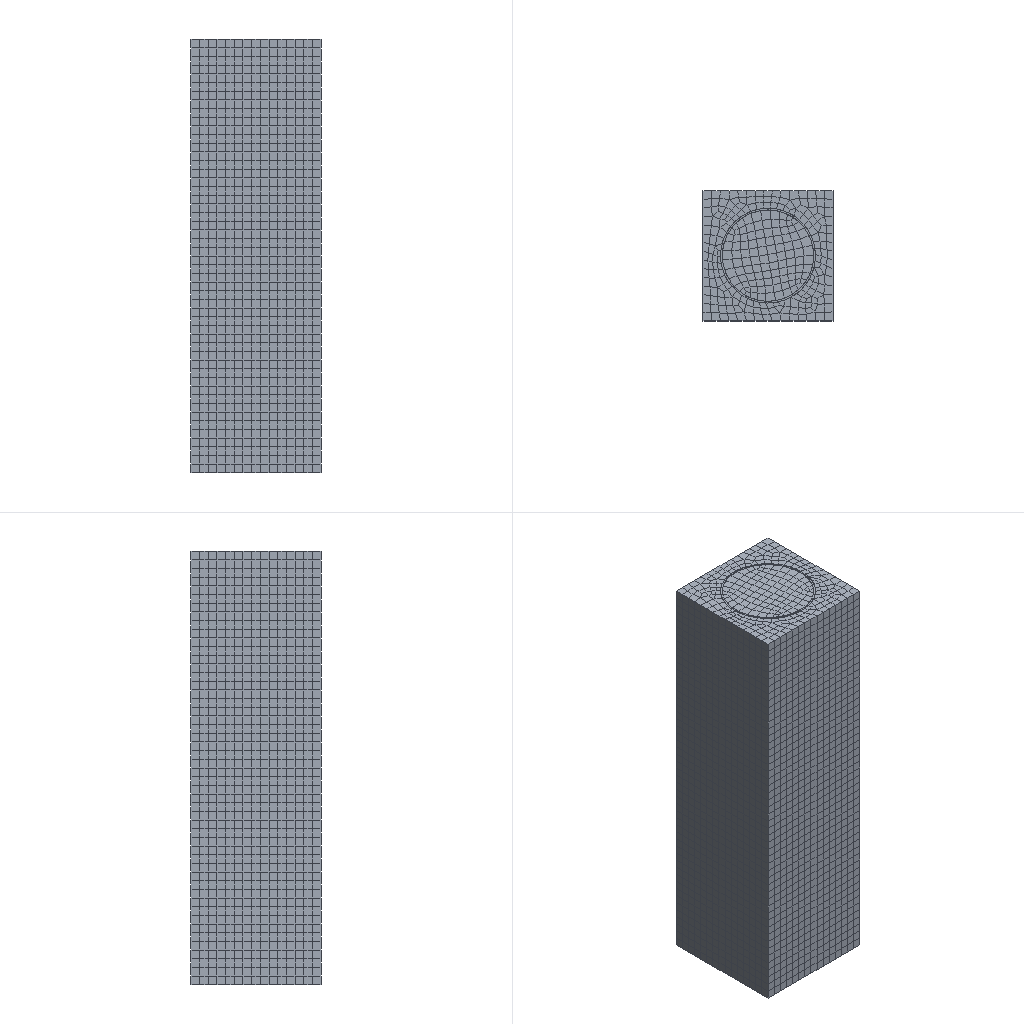Simulation study | abaqus
Set-up summary:
category,name,step,type,value,unit,region
solver,abaqus
solver,version,,,Abaqus/Explicit 2020
units,not stated in the deck,,not stated
analysis,deck,,transient,transient
load_step,Step-1,Step-1,transient,nlgeom=True
contact,interactions,,,general=1 pairs=0 ties=0
load_step,requested,,,1
mesh,nodes,,,23143
mesh,elements,,,17443
element_type,T3D2,,truss,743
element_type,C3D8R,,solid,16700
load,load commands in deck,,count,1
bc,support commands in deck,,count,7
material,CON,,in results
material,GUJIN,,in results
material,SHUJIN,,in results
material,STEEL,,in results
check,setup vs results,,match,"per instance, exact: element labels, types and connectivity; labels of the nodes the elements use; coordinates of those nodes at SINGLE_PRECISION in 4 of 4 instance(s)"
Abaqus input file, long lists of numbers shortened:
*Heading
** Job name: Job-1 Model name: Model-1
** Generated by: Abaqus/CAE 2020
*Preprint, echo=NO, model=NO, history=NO, contact=NO
**
** PARTS
**
*Part, name=con-final
*Node
      1,   226.771,  -228.08,           0.
      2,   251.522,  -191.03,           0.
** (12544 more lines like these left out)
*Element, type=C3D8R
   1,    50,    49,   245,   149,   296,   295,   491,   395
   2,   177,   245,   147,   213,   423,   491,   393,   459
** (9648 more lines like these left out)
*Nset, nset=Set-6, generate
     1,  12546,      1
*Elset, elset=Set-6, generate
    1,  9650,     1
** Section: con
*Solid Section, elset=Set-6, material=con
,
*End Part
**
*Part, name=jin-fianl
*Node
      1,          25.,        -275.,         930.
      2,          25.,         -25.,         930.
** (701 more lines like these left out)
*Element, type=T3D2
 1,  2, 53
 2, 53, 54
** (741 more lines like these left out)
*Nset, nset=Set-1
   1,   2,   3,   4,   5,   6,   7,   8,   9,  10,  11,  12,  13,  14,  15,  16
  17,  18,  19,  20,  21,  22,  23,  24,  25,  26,  27,  28,  29,  30,  31,  32
** (9 more lines like these left out)
*Elset, elset=Set-1
  27,  28,  29,  30,  44,  45,  46,  47,  61,  62,  63,  64,  91,  92,  93,  94
 108, 109, 110, 111, 125, 126, 127, 128, 155, 156, 157, 158, 172, 173, 174, 175
** (9 more lines like these left out)
*Nset, nset=Set-2
   1,   2,   3,   4,   5,   6,   7,   8,   9,  10,  11,  12,  13,  14,  15,  16
  17,  18,  19,  20,  21,  22,  23,  24,  25,  26,  28,  29,  30,  32,  33,  34
** (34 more lines like these left out)
*Elset, elset=Set-2
   1,   2,   3,   4,   5,   6,   7,   8,   9,  10,  11,  12,  13,  14,  15,  16
  17,  18,  19,  20,  21,  22,  23,  24,  25,  26,  31,  32,  33,  34,  35,  36
** (34 more lines like these left out)
** Section: gujin
*Solid Section, elset=Set-2, material=gujin
28.26,
** Section: shujin
*Solid Section, elset=Set-1, material=shujin
78.5,
*End Part
**
*Part, name=nc
*Node
      1,   2.953,  -16.812,           0.
      2,   105.493,   1.202,           0.
** (6322 more lines like these left out)
*Element, type=C3D8R
   1,  130,  131,  184,  183,    6,    7,   60,   59
   2,  131,  132,  185,  184,    7,    8,   61,   60
** (5298 more lines like these left out)
*Nset, nset=Set-2, generate
    1,  6324,     1
*Elset, elset=Set-2, generate
    1,  5300,     1
** Section: con
*Solid Section, elset=Set-2, material=con
,
*End Part
**
*Part, name=tube
*Node
      1,    89.911,   -55.192,           0.
      2,   93.321,  -57.284,           0.
** (3568 more lines like these left out)
*Element, type=C3D8R
   1,   71,   72,   82,   88,    1,    2,   12,   18
   2,   88,   82,   83,   87,   18,   12,   13,   17
** (1748 more lines like these left out)
*Nset, nset=Set-1, generate
    1,  3570,     1
*Elset, elset=Set-1, generate
    1,  1750,     1
** Section: tube
*Solid Section, elset=Set-1, material=steel
,
*End Part
**
**
** ASSEMBLY
**
*Assembly, name=Assembly
**
*Instance, name=tube-1, part=tube
        150.,        -150.,           0.
*End Instance
**
*Instance, name=con-final-1, part=con-final
*End Instance
**
*Instance, name=jin-fianl-1, part=jin-fianl
*End Instance
**
*Instance, name=nc-1, part=nc
        150.,        -150.,           0.
*End Instance
**
*Node
      1,         150.,        -150.,           0.
*Nset, nset=Set-1, instance=tube-1, generate
 3501,  3570,     1
*Nset, nset=Set-1, instance=con-final-1, generate
 12301,  12546,      1
*Nset, nset=Set-1, instance=nc-1, generate
 6201,  6324,     1
*Elset, elset=Set-1, instance=tube-1, generate
 1716,  1750,     1
*Elset, elset=Set-1, instance=con-final-1, generate
 9458,  9650,     1
*Elset, elset=Set-1, instance=nc-1, generate
 5195,  5300,     1
*Nset, nset=Set-3
 1,
*Nset, nset=m_Set-2
 1,
*Nset, nset=m_Set-4, instance=jin-fianl-1, generate
   1,  703,    1
*Elset, elset=m_Set-4, instance=jin-fianl-1, generate
   1,  743,    1
*Nset, nset=s_Set-4, instance=con-final-1, generate
     1,  12546,      1
*Elset, elset=s_Set-4, instance=con-final-1, generate
    1,  9650,     1
*Elset, elset=_s_Surf-1_S2, internal, instance=tube-1, generate
  1,  35,   1
*Elset, elset=_s_Surf-1_S2, internal, instance=nc-1, generate
   1,  106,    1
*Elset, elset=_s_Surf-1_S1, internal, instance=con-final-1, generate
   1,  193,    1
*Surface, type=ELEMENT, name=s_Surf-1
_s_Surf-1_S2, S2
_s_Surf-1_S1, S1
** Constraint: Constraint-1
*Coupling, constraint name=Constraint-1, ref node=m_Set-2, surface=s_Surf-1
*Kinematic
** Constraint: Constraint-2
*Embedded Element, host elset=s_Set-4
m_Set-4
*End Assembly
*Amplitude, name=Amp-1
             0.,              0.,            0.01,              1.
**
** MATERIALS
**
*Material, name=con
*Density
 2.5e-09,
*Elastic
32500., 0.2
*Concrete Damaged Plasticity
30.,   0.1,  1.16, 0.667,  0.01
*Concrete Compression Hardening
 31.839,          0.
  35.238, 0.0001688
  37.656, 0.0002734
 39.058, 0.0004092
    39.5, 0.0005746
 38.815, 0.0007747
 37.101,  0.001006
  34.823,  0.001256
 32.332,  0.001511
 29.849,  0.001767
 27.497,  0.002018
 25.334,   0.002263
 23.376,  0.002503
 21.619,  0.002736
 20.051,  0.002963
 18.651,  0.003185
 17.402,  0.003403
 16.285,  0.003616
 15.284,  0.003826
 14.385,   0.004032
 13.573,  0.004236
 12.839,  0.004438
 12.173,  0.004637
 11.567,   0.004835
  11.013,  0.005031
*Concrete Tension Stiffening
  2.09,       0.
   2.4, 8.74e-06
  2.67, 1.23e-05
  2.86, 1.81e-05
  2.94, 2.75e-05
   2.8, 4.37e-05
  2.55, 6.31e-05
   2.3, 8.27e-05
  2.07, 0.000102
  1.86,  0.00012
  1.69, 0.000137
  1.55, 0.000153
  1.42, 0.000169
  1.31, 0.000184
  1.22, 0.000198
  1.14, 0.000213
  1.07, 0.000227
  1.01,  0.00024
 0.956, 0.000254
 0.908, 0.000267
 0.864,  0.00028
 0.825, 0.000293
 0.789, 0.000306
 0.757, 0.000319
 0.727, 0.000332
*Concrete Compression Damage
        0.,          0.
 0.06977, 0.0001688
  0.1005, 0.0002734
  0.1363, 0.0004092
  0.176, 0.0005746
  0.2212, 0.0007747
  0.271,  0.001006
  0.3214,  0.001256
  0.3699,  0.001511
  0.4151,  0.001767
  0.4565,  0.002018
  0.4939,   0.002263
  0.5275,  0.002503
   0.5577,  0.002736
  0.5849,  0.002963
   0.6093,  0.003185
  0.6313,  0.003403
  0.6511,  0.003616
  0.6691,  0.003826
  0.6855,   0.004032
  0.7004,  0.004236
  0.7141,  0.004438
  0.7266,  0.004637
  0.7382,   0.004835
  0.7488,  0.005031
  0.7586,  0.005226
  0.7678,  0.005419
  0.7763,  0.005611
  0.7842,  0.005802
  0.7915,  0.005993
  0.7984,  0.006182
  0.8049,  0.006371
  0.811,  0.006559
  0.8167,  0.006747
  0.8221,  0.006933
  0.8627,  0.008781
  0.8884,   0.01061
  0.906,   0.01242
  0.9188,   0.01423
  0.9286,   0.01603
** (21 more lines like these left out)
*Concrete Tension Damage, compression recovery=0.45
     0.,       0.
 0.0544, 8.74e-06
 0.0674, 1.23e-05
 0.0893, 1.81e-05
  0.124, 2.75e-05
  0.186, 4.37e-05
  0.255, 6.31e-05
  0.321, 8.27e-05
   0.38, 0.000102
  0.431,  0.00012
  0.475, 0.000137
  0.513, 0.000153
  0.546, 0.000169
  0.575, 0.000184
  0.601, 0.000198
  0.623, 0.000213
  0.643, 0.000227
  0.661,  0.00024
  0.678, 0.000254
  0.692, 0.000267
  0.706,  0.00028
  0.718, 0.000293
  0.729, 0.000306
  0.739, 0.000319
  0.749, 0.000332
  0.757, 0.000344
  0.765, 0.000357
  0.773, 0.000369
   0.78, 0.000382
  0.787, 0.000394
  0.793, 0.000407
  0.799, 0.000419
  0.804, 0.000431
  0.809, 0.000443
  0.814, 0.000456
  0.851, 0.000577
  0.875, 0.000697
  0.892, 0.000816
  0.905, 0.000935
  0.915,  0.00105
** (31 more lines like these left out)
*Material, name=gujin
*Density
 7.85e-09,
*Elastic
206000., 0.3
*Plastic
475.,     0.
605., 0.0602
*Material, name=shujin
*Density
 7.85e-09,
*Elastic
206000., 0.3
*Plastic
485.,     0.
625., 0.0649
*Material, name=steel
*Density
 7.85e-09,
*Elastic
206000., 0.3
*Plastic
376.,     0.
525., 0.0698
**
** INTERACTION PROPERTIES
**
*Surface Interaction, name=IntProp-1
*Friction
 0.1,
*Surface Behavior, pressure-overclosure=HARD
** ----------------------------------------------------------------
**
** STEP: Step-1
**
*Step, name=Step-1, nlgeom=YES
*Dynamic, Explicit
, 0.01
*Bulk Viscosity
0.06, 1.2
**
** BOUNDARY CONDITIONS
**
** Name: BC-1 Type: 对称/反对称/完全固定
*Boundary
Set-1, ENCASTRE
** Name: [REDACTED] : Displacement/rotation angle
*Boundary, amplitude=Amp-1
Set-3, 1, 1
Set-3, 2, 2
Set-3, 3, 3, 50.
Set-3, 4, 4
Set-3, 5, 5
Set-3, 6, 6
**
** INTERACTIONS
**
** Interaction: Int-1
*Contact, op=NEW
*Contact Inclusions, ALL EXTERIOR
*Contact Property Assignment
 ,  , IntProp-1
**
** OUTPUT REQUESTS
**
*Restart, write, number interval=1, time marks=NO
**
** FIELD OUTPUT: F-Output-1
**
*Output, field, number interval=50
*Node Output
A, CF, RF, RM, RT, U, V
*Element Output, directions=YES
DAMAGEC, DAMAGET, E, EVF, LE, MISES, MISESMAX, MISESONLY, P, PE, PEEQ, PEEQMAX, PEEQT, PEEQVAVG, PEMAG, PEVAVG
S, SDEG, SF, SSAVG, SVAVG, YIELDPOT
*Contact Output
CDISP, CFORCE, CSTRESS, FSLIP, FSLIPR, PPRESS
**
** HISTORY OUTPUT: H-Output-1
**
*Output, history, time interval=1e-07
*Node Output, nset=Set-3
RF3, U3
*End Step
Results summary:
result,step,Step-1,completed,increments=17212 time=0.01/0.01
result,analysis,,,transient
result,last_loadstep,,,1
result,analysis steps,,count,1
result,primary field,,,U
result,reaction total,,FX,-3554.903,model units
result,reaction total,,FY,1692.277,model units
result,reaction total,,FZ,-91990.286,model units